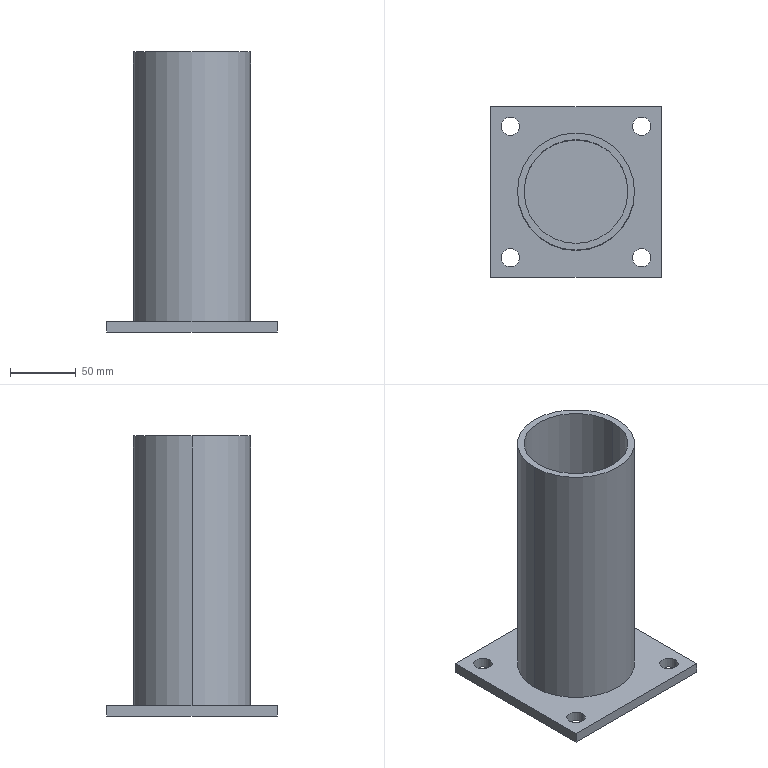Part | SolidWorks | features Extrusion 1, WeldMemberFeat 1, WeldmentFeature 1 | 2 solids | 20 faces | box 130 x 130 x 213 mm | volume 400765 mm3 | cylinder 12 | plane 8 | commonest cylinder face diameters 14 x8 79 x2 89 x2
STEP:
#1=CARTESIAN_POINT('',(-57.,-50.,8.));
#2=VERTEX_POINT('',#1);
#3=CARTESIAN_POINT('',(-43.,-50.,8.));
#4=VERTEX_POINT('',#3);
#5=CARTESIAN_POINT('',(-50.,-50.,8.));
#6=DIRECTION('',(0.,0.,1.));
#7=DIRECTION('',(-1.,0.,0.));
#8=AXIS2_PLACEMENT_3D('',#5,#6,#7);
#9=CIRCLE('',#8,7.);
#10=EDGE_CURVE('',#2,#4,#9,.T.);
#11=ORIENTED_EDGE('',*,*,#10,.T.);
#12=CARTESIAN_POINT('',(-43.,-50.,0.));
#13=VERTEX_POINT('',#12);
#14=CARTESIAN_POINT('',(-43.,-50.,8.));
#15=DIRECTION('',(0.,0.,-1.));
#16=VECTOR('',#15,1000.);
#17=LINE('',#14,#16);
#18=EDGE_CURVE('',#4,#13,#17,.T.);
#19=ORIENTED_EDGE('',*,*,#18,.T.);
#20=CARTESIAN_POINT('',(-57.,-50.,0.));
#21=VERTEX_POINT('',#20);
#22=CARTESIAN_POINT('',(-50.,-50.,0.));
#23=DIRECTION('',(0.,0.,1.));
#24=DIRECTION('',(-1.,0.,0.));
#25=AXIS2_PLACEMENT_3D('',#22,#23,#24);
#26=CIRCLE('',#25,7.);
#27=EDGE_CURVE('',#21,#13,#26,.T.);
#28=ORIENTED_EDGE('',*,*,#27,.F.);
#29=CARTESIAN_POINT('',(-57.,-50.,8.));
#30=DIRECTION('',(0.,0.,-1.));
#31=VECTOR('',#30,1000.);
#32=LINE('',#29,#31);
#33=EDGE_CURVE('',#2,#21,#32,.T.);
#34=ORIENTED_EDGE('',*,*,#33,.F.);
#35=EDGE_LOOP('',(#11,#19,#28,#34));
#36=FACE_OUTER_BOUND('',#35,.T.);
#37=CARTESIAN_POINT('',(-50.,-50.,8.));
#38=DIRECTION('',(0.,0.,-1.));
#39=DIRECTION('',(-1.,0.,0.));
#40=AXIS2_PLACEMENT_3D('',#37,#38,#39);
#41=CYLINDRICAL_SURFACE('',#40,7.);
#42=ADVANCED_FACE('',(#36),#41,.F.);
#43=CARTESIAN_POINT('',(43.,-50.,8.));
#44=VERTEX_POINT('',#43);
#45=CARTESIAN_POINT('',(57.,-50.,8.));
#46=VERTEX_POINT('',#45);
#47=CARTESIAN_POINT('',(50.,-50.,8.));
#48=DIRECTION('',(0.,0.,1.));
#49=DIRECTION('',(1.,0.,0.));
#50=AXIS2_PLACEMENT_3D('',#47,#48,#49);
#51=CIRCLE('',#50,7.);
#52=EDGE_CURVE('',#44,#46,#51,.T.);
#53=ORIENTED_EDGE('',*,*,#52,.T.);
#54=CARTESIAN_POINT('',(57.,-50.,0.));
#55=VERTEX_POINT('',#54);
#56=CARTESIAN_POINT('',(57.,-50.,8.));
#57=DIRECTION('',(0.,0.,-1.));
#58=VECTOR('',#57,1000.);
#59=LINE('',#56,#58);
#60=EDGE_CURVE('',#46,#55,#59,.T.);
#61=ORIENTED_EDGE('',*,*,#60,.T.);
#62=CARTESIAN_POINT('',(43.,-50.,0.));
#63=VERTEX_POINT('',#62);
#64=CARTESIAN_POINT('',(50.,-50.,0.));
#65=DIRECTION('',(0.,0.,1.));
#66=DIRECTION('',(1.,0.,0.));
#67=AXIS2_PLACEMENT_3D('',#64,#65,#66);
#68=CIRCLE('',#67,7.);
#69=EDGE_CURVE('',#63,#55,#68,.T.);
#70=ORIENTED_EDGE('',*,*,#69,.F.);
#71=CARTESIAN_POINT('',(43.,-50.,8.));
#72=DIRECTION('',(0.,0.,-1.));
#73=VECTOR('',#72,1000.);
#74=LINE('',#71,#73);
#75=EDGE_CURVE('',#44,#63,#74,.T.);
#76=ORIENTED_EDGE('',*,*,#75,.F.);
#77=EDGE_LOOP('',(#53,#61,#70,#76));
#78=FACE_OUTER_BOUND('',#77,.T.);
#79=CARTESIAN_POINT('',(50.,-50.,8.));
#80=DIRECTION('',(0.,0.,-1.));
#81=DIRECTION('',(-1.,0.,0.));
#82=AXIS2_PLACEMENT_3D('',#79,#80,#81);
#83=CYLINDRICAL_SURFACE('',#82,7.);
#84=ADVANCED_FACE('',(#78),#83,.F.);
#85=CARTESIAN_POINT('',(43.,50.,8.));
#86=VERTEX_POINT('',#85);
#87=CARTESIAN_POINT('',(57.,50.,8.));
#88=VERTEX_POINT('',#87);
#89=CARTESIAN_POINT('',(50.,50.,8.));
#90=DIRECTION('',(0.,0.,1.));
#91=DIRECTION('',(-1.,0.,0.));
#92=AXIS2_PLACEMENT_3D('',#89,#90,#91);
#93=CIRCLE('',#92,7.);
#94=EDGE_CURVE('',#86,#88,#93,.T.);
#95=ORIENTED_EDGE('',*,*,#94,.T.);
#96=CARTESIAN_POINT('',(57.,50.,0.));
#97=VERTEX_POINT('',#96);
#98=CARTESIAN_POINT('',(57.,50.,8.));
#99=DIRECTION('',(0.,0.,-1.));
#100=VECTOR('',#99,1000.);
#101=LINE('',#98,#100);
#102=EDGE_CURVE('',#88,#97,#101,.T.);
#103=ORIENTED_EDGE('',*,*,#102,.T.);
#104=CARTESIAN_POINT('',(43.,50.,0.));
#105=VERTEX_POINT('',#104);
#106=CARTESIAN_POINT('',(50.,50.,0.));
#107=DIRECTION('',(0.,0.,1.));
#108=DIRECTION('',(-1.,0.,0.));
#109=AXIS2_PLACEMENT_3D('',#106,#107,#108);
#110=CIRCLE('',#109,7.);
#111=EDGE_CURVE('',#105,#97,#110,.T.);
#112=ORIENTED_EDGE('',*,*,#111,.F.);
#113=CARTESIAN_POINT('',(43.,50.,8.));
#114=DIRECTION('',(0.,0.,-1.));
#115=VECTOR('',#114,1000.);
#116=LINE('',#113,#115);
#117=EDGE_CURVE('',#86,#105,#116,.T.);
#118=ORIENTED_EDGE('',*,*,#117,.F.);
#119=EDGE_LOOP('',(#95,#103,#112,#118));
#120=FACE_OUTER_BOUND('',#119,.T.);
#121=CARTESIAN_POINT('',(50.,50.,8.));
#122=DIRECTION('',(0.,0.,-1.));
#123=DIRECTION('',(-1.,0.,0.));
#124=AXIS2_PLACEMENT_3D('',#121,#122,#123);
#125=CYLINDRICAL_SURFACE('',#124,7.);
#126=ADVANCED_FACE('',(#120),#125,.F.);
#127=CARTESIAN_POINT('',(-57.,50.,8.));
#128=VERTEX_POINT('',#127);
#129=CARTESIAN_POINT('',(-43.,50.,8.));
#130=VERTEX_POINT('',#129);
#131=CARTESIAN_POINT('',(-50.,50.,8.));
#132=DIRECTION('',(0.,0.,1.));
#133=DIRECTION('',(1.,0.,0.));
#134=AXIS2_PLACEMENT_3D('',#131,#132,#133);
#135=CIRCLE('',#134,7.);
#136=EDGE_CURVE('',#128,#130,#135,.T.);
#137=ORIENTED_EDGE('',*,*,#136,.T.);
#138=CARTESIAN_POINT('',(-43.,50.,0.));
#139=VERTEX_POINT('',#138);
#140=CARTESIAN_POINT('',(-43.,50.,8.));
#141=DIRECTION('',(0.,0.,-1.));
#142=VECTOR('',#141,1000.);
#143=LINE('',#140,#142);
#144=EDGE_CURVE('',#130,#139,#143,.T.);
#145=ORIENTED_EDGE('',*,*,#144,.T.);
#146=CARTESIAN_POINT('',(-57.,50.,0.));
#147=VERTEX_POINT('',#146);
#148=CARTESIAN_POINT('',(-50.,50.,0.));
#149=DIRECTION('',(0.,0.,1.));
#150=DIRECTION('',(1.,0.,0.));
#151=AXIS2_PLACEMENT_3D('',#148,#149,#150);
#152=CIRCLE('',#151,7.);
#153=EDGE_CURVE('',#147,#139,#152,.T.);
#154=ORIENTED_EDGE('',*,*,#153,.F.);
#155=CARTESIAN_POINT('',(-57.,50.,8.));
#156=DIRECTION('',(0.,0.,-1.));
#157=VECTOR('',#156,1000.);
#158=LINE('',#155,#157);
#159=EDGE_CURVE('',#128,#147,#158,.T.);
#160=ORIENTED_EDGE('',*,*,#159,.F.);
#161=EDGE_LOOP('',(#137,#145,#154,#160));
#162=FACE_OUTER_BOUND('',#161,.T.);
#163=CARTESIAN_POINT('',(-50.,50.,8.));
#164=DIRECTION('',(0.,0.,-1.));
#165=DIRECTION('',(-1.,0.,0.));
#166=AXIS2_PLACEMENT_3D('',#163,#164,#165);
#167=CYLINDRICAL_SURFACE('',#166,7.);
#168=ADVANCED_FACE('',(#162),#167,.F.);
#169=ORIENTED_EDGE('',*,*,#52,.F.);
#170=CARTESIAN_POINT('',(50.,-50.,8.));
#171=DIRECTION('',(0.,0.,1.));
#172=DIRECTION('',(1.,0.,0.));
#173=AXIS2_PLACEMENT_3D('',#170,#171,#172);
#174=CIRCLE('',#173,7.);
#175=EDGE_CURVE('',#46,#44,#174,.T.);
#176=ORIENTED_EDGE('',*,*,#175,.F.);
#177=EDGE_LOOP('',(#169,#176));
#178=FACE_BOUND('',#177,.T.);
#179=ORIENTED_EDGE('',*,*,#136,.F.);
#180=CARTESIAN_POINT('',(-50.,50.,8.));
#181=DIRECTION('',(0.,0.,1.));
#182=DIRECTION('',(1.,0.,0.));
#183=AXIS2_PLACEMENT_3D('',#180,#181,#182);
#184=CIRCLE('',#183,7.);
#185=EDGE_CURVE('',#130,#128,#184,.T.);
#186=ORIENTED_EDGE('',*,*,#185,.F.);
#187=EDGE_LOOP('',(#179,#186));
#188=FACE_BOUND('',#187,.T.);
#189=CARTESIAN_POINT('',(-65.,65.,8.));
#190=VERTEX_POINT('',#189);
#191=CARTESIAN_POINT('',(-65.,-65.,8.));
#192=VERTEX_POINT('',#191);
#193=CARTESIAN_POINT('',(-65.,-65.,8.));
#194=DIRECTION('',(0.,-1.,0.));
#195=VECTOR('',#194,1000.);
#196=LINE('',#193,#195);
#197=EDGE_CURVE('',#190,#192,#196,.T.);
#198=ORIENTED_EDGE('',*,*,#197,.T.);
#199=CARTESIAN_POINT('',(65.,-65.,8.));
#200=VERTEX_POINT('',#199);
#201=CARTESIAN_POINT('',(65.,-65.,8.));
#202=DIRECTION('',(1.,0.,0.));
#203=VECTOR('',#202,1000.);
#204=LINE('',#201,#203);
#205=EDGE_CURVE('',#192,#200,#204,.T.);
#206=ORIENTED_EDGE('',*,*,#205,.T.);
#207=CARTESIAN_POINT('',(65.,65.,8.));
#208=VERTEX_POINT('',#207);
#209=CARTESIAN_POINT('',(65.,-65.,8.));
#210=DIRECTION('',(0.,1.,0.));
#211=VECTOR('',#210,1000.);
#212=LINE('',#209,#211);
#213=EDGE_CURVE('',#200,#208,#212,.T.);
#214=ORIENTED_EDGE('',*,*,#213,.T.);
#215=CARTESIAN_POINT('',(65.,65.,8.));
#216=DIRECTION('',(-1.,0.,0.));
#217=VECTOR('',#216,1000.);
#218=LINE('',#215,#217);
#219=EDGE_CURVE('',#208,#190,#218,.T.);
#220=ORIENTED_EDGE('',*,*,#219,.T.);
#221=EDGE_LOOP('',(#198,#206,#214,#220));
#222=FACE_OUTER_BOUND('',#221,.T.);
#223=ORIENTED_EDGE('',*,*,#94,.F.);
#224=CARTESIAN_POINT('',(50.,50.,8.));
#225=DIRECTION('',(0.,0.,1.));
#226=DIRECTION('',(-1.,0.,0.));
#227=AXIS2_PLACEMENT_3D('',#224,#225,#226);
#228=CIRCLE('',#227,7.);
#229=EDGE_CURVE('',#88,#86,#228,.T.);
#230=ORIENTED_EDGE('',*,*,#229,.F.);
#231=EDGE_LOOP('',(#223,#230));
#232=FACE_BOUND('',#231,.T.);
#233=ORIENTED_EDGE('',*,*,#10,.F.);
#234=CARTESIAN_POINT('',(-50.,-50.,8.));
#235=DIRECTION('',(0.,0.,1.));
#236=DIRECTION('',(-1.,0.,0.));
#237=AXIS2_PLACEMENT_3D('',#234,#235,#236);
#238=CIRCLE('',#237,7.);
#239=EDGE_CURVE('',#4,#2,#238,.T.);
#240=ORIENTED_EDGE('',*,*,#239,.F.);
#241=EDGE_LOOP('',(#233,#240));
#242=FACE_BOUND('',#241,.T.);
#243=CARTESIAN_POINT('',(0.,0.,8.));
#244=DIRECTION('',(0.,0.,1.));
#245=DIRECTION('',(1.,0.,0.));
#246=AXIS2_PLACEMENT_3D('',#243,#244,#245);
#247=PLANE('',#246);
#248=ADVANCED_FACE('',(#178,#188,#222,#232,#242),#247,.T.);
#249=CARTESIAN_POINT('',(-65.,65.,0.));
#250=VERTEX_POINT('',#249);
#251=CARTESIAN_POINT('',(-65.,-65.,0.));
#252=VERTEX_POINT('',#251);
#253=CARTESIAN_POINT('',(-65.,-65.,0.));
#254=DIRECTION('',(0.,-1.,0.));
#255=VECTOR('',#254,1000.);
#256=LINE('',#253,#255);
#257=EDGE_CURVE('',#250,#252,#256,.T.);
#258=ORIENTED_EDGE('',*,*,#257,.F.);
#259=CARTESIAN_POINT('',(65.,65.,0.));
#260=VERTEX_POINT('',#259);
#261=CARTESIAN_POINT('',(65.,65.,0.));
#262=DIRECTION('',(-1.,0.,0.));
#263=VECTOR('',#262,1000.);
#264=LINE('',#261,#263);
#265=EDGE_CURVE('',#260,#250,#264,.T.);
#266=ORIENTED_EDGE('',*,*,#265,.F.);
#267=CARTESIAN_POINT('',(65.,-65.,0.));
#268=VERTEX_POINT('',#267);
#269=CARTESIAN_POINT('',(65.,-65.,0.));
#270=DIRECTION('',(0.,1.,0.));
#271=VECTOR('',#270,1000.);
#272=LINE('',#269,#271);
#273=EDGE_CURVE('',#268,#260,#272,.T.);
#274=ORIENTED_EDGE('',*,*,#273,.F.);
#275=CARTESIAN_POINT('',(65.,-65.,0.));
#276=DIRECTION('',(1.,0.,0.));
#277=VECTOR('',#276,1000.);
#278=LINE('',#275,#277);
#279=EDGE_CURVE('',#252,#268,#278,.T.);
#280=ORIENTED_EDGE('',*,*,#279,.F.);
#281=EDGE_LOOP('',(#258,#266,#274,#280));
#282=FACE_OUTER_BOUND('',#281,.T.);
#283=ORIENTED_EDGE('',*,*,#153,.T.);
#284=CARTESIAN_POINT('',(-50.,50.,0.));
#285=DIRECTION('',(0.,0.,1.));
#286=DIRECTION('',(1.,0.,0.));
#287=AXIS2_PLACEMENT_3D('',#284,#285,#286);
#288=CIRCLE('',#287,7.);
#289=EDGE_CURVE('',#139,#147,#288,.T.);
#290=ORIENTED_EDGE('',*,*,#289,.T.);
#291=EDGE_LOOP('',(#283,#290));
#292=FACE_BOUND('',#291,.T.);
#293=ORIENTED_EDGE('',*,*,#111,.T.);
#294=CARTESIAN_POINT('',(50.,50.,0.));
#295=DIRECTION('',(0.,0.,1.));
#296=DIRECTION('',(-1.,0.,0.));
#297=AXIS2_PLACEMENT_3D('',#294,#295,#296);
#298=CIRCLE('',#297,7.);
#299=EDGE_CURVE('',#97,#105,#298,.T.);
#300=ORIENTED_EDGE('',*,*,#299,.T.);
#301=EDGE_LOOP('',(#293,#300));
#302=FACE_BOUND('',#301,.T.);
#303=ORIENTED_EDGE('',*,*,#69,.T.);
#304=CARTESIAN_POINT('',(50.,-50.,0.));
#305=DIRECTION('',(0.,0.,1.));
#306=DIRECTION('',(1.,0.,0.));
#307=AXIS2_PLACEMENT_3D('',#304,#305,#306);
#308=CIRCLE('',#307,7.);
#309=EDGE_CURVE('',#55,#63,#308,.T.);
#310=ORIENTED_EDGE('',*,*,#309,.T.);
#311=EDGE_LOOP('',(#303,#310));
#312=FACE_BOUND('',#311,.T.);
#313=ORIENTED_EDGE('',*,*,#27,.T.);
#314=CARTESIAN_POINT('',(-50.,-50.,0.));
#315=DIRECTION('',(0.,0.,1.));
#316=DIRECTION('',(-1.,0.,0.));
#317=AXIS2_PLACEMENT_3D('',#314,#315,#316);
#318=CIRCLE('',#317,7.);
#319=EDGE_CURVE('',#13,#21,#318,.T.);
#320=ORIENTED_EDGE('',*,*,#319,.T.);
#321=EDGE_LOOP('',(#313,#320));
#322=FACE_BOUND('',#321,.T.);
#323=CARTESIAN_POINT('',(0.,0.,0.));
#324=DIRECTION('',(0.,0.,1.));
#325=DIRECTION('',(1.,0.,0.));
#326=AXIS2_PLACEMENT_3D('',#323,#324,#325);
#327=PLANE('',#326);
#328=ADVANCED_FACE('',(#282,#292,#302,#312,#322),#327,.F.);
#329=ORIENTED_EDGE('',*,*,#257,.T.);
#330=CARTESIAN_POINT('',(-65.,-65.,8.));
#331=DIRECTION('',(0.,0.,-1.));
#332=VECTOR('',#331,1000.);
#333=LINE('',#330,#332);
#334=EDGE_CURVE('',#192,#252,#333,.T.);
#335=ORIENTED_EDGE('',*,*,#334,.F.);
#336=ORIENTED_EDGE('',*,*,#197,.F.);
#337=CARTESIAN_POINT('',(-65.,65.,8.));
#338=DIRECTION('',(0.,0.,-1.));
#339=VECTOR('',#338,1000.);
#340=LINE('',#337,#339);
#341=EDGE_CURVE('',#190,#250,#340,.T.);
#342=ORIENTED_EDGE('',*,*,#341,.T.);
#343=EDGE_LOOP('',(#329,#335,#336,#342));
#344=FACE_OUTER_BOUND('',#343,.T.);
#345=CARTESIAN_POINT('',(-65.,-65.,8.));
#346=DIRECTION('',(1.,0.,0.));
#347=DIRECTION('',(0.,0.,-1.));
#348=AXIS2_PLACEMENT_3D('',#345,#346,#347);
#349=PLANE('',#348);
#350=ADVANCED_FACE('',(#344),#349,.F.);
#351=ORIENTED_EDGE('',*,*,#279,.T.);
#352=CARTESIAN_POINT('',(65.,-65.,8.));
#353=DIRECTION('',(0.,0.,-1.));
#354=VECTOR('',#353,1000.);
#355=LINE('',#352,#354);
#356=EDGE_CURVE('',#200,#268,#355,.T.);
#357=ORIENTED_EDGE('',*,*,#356,.F.);
#358=ORIENTED_EDGE('',*,*,#205,.F.);
#359=ORIENTED_EDGE('',*,*,#334,.T.);
#360=EDGE_LOOP('',(#351,#357,#358,#359));
#361=FACE_OUTER_BOUND('',#360,.T.);
#362=CARTESIAN_POINT('',(65.,-65.,8.));
#363=DIRECTION('',(0.,1.,0.));
#364=DIRECTION('',(-1.,0.,0.));
#365=AXIS2_PLACEMENT_3D('',#362,#363,#364);
#366=PLANE('',#365);
#367=ADVANCED_FACE('',(#361),#366,.F.);
#368=ORIENTED_EDGE('',*,*,#273,.T.);
#369=CARTESIAN_POINT('',(65.,65.,8.));
#370=DIRECTION('',(0.,0.,-1.));
#371=VECTOR('',#370,1000.);
#372=LINE('',#369,#371);
#373=EDGE_CURVE('',#208,#260,#372,.T.);
#374=ORIENTED_EDGE('',*,*,#373,.F.);
#375=ORIENTED_EDGE('',*,*,#213,.F.);
#376=ORIENTED_EDGE('',*,*,#356,.T.);
#377=EDGE_LOOP('',(#368,#374,#375,#376));
#378=FACE_OUTER_BOUND('',#377,.T.);
#379=CARTESIAN_POINT('',(65.,-65.,8.));
#380=DIRECTION('',(-1.,0.,0.));
#381=DIRECTION('',(0.,0.,1.));
#382=AXIS2_PLACEMENT_3D('',#379,#380,#381);
#383=PLANE('',#382);
#384=ADVANCED_FACE('',(#378),#383,.F.);
#385=ORIENTED_EDGE('',*,*,#265,.T.);
#386=ORIENTED_EDGE('',*,*,#341,.F.);
#387=ORIENTED_EDGE('',*,*,#219,.F.);
#388=ORIENTED_EDGE('',*,*,#373,.T.);
#389=EDGE_LOOP('',(#385,#386,#387,#388));
#390=FACE_OUTER_BOUND('',#389,.T.);
#391=CARTESIAN_POINT('',(65.,65.,8.));
#392=DIRECTION('',(0.,-1.,0.));
#393=DIRECTION('',(0.,0.,-1.));
#394=AXIS2_PLACEMENT_3D('',#391,#392,#393);
#395=PLANE('',#394);
#396=ADVANCED_FACE('',(#390),#395,.F.);
#397=ORIENTED_EDGE('',*,*,#144,.F.);
#398=ORIENTED_EDGE('',*,*,#185,.T.);
#399=ORIENTED_EDGE('',*,*,#159,.T.);
#400=ORIENTED_EDGE('',*,*,#289,.F.);
#401=EDGE_LOOP('',(#397,#398,#399,#400));
#402=FACE_OUTER_BOUND('',#401,.T.);
#403=CARTESIAN_POINT('',(-50.,50.,8.));
#404=DIRECTION('',(0.,0.,-1.));
#405=DIRECTION('',(-1.,0.,0.));
#406=AXIS2_PLACEMENT_3D('',#403,#404,#405);
#407=CYLINDRICAL_SURFACE('',#406,7.);
#408=ADVANCED_FACE('',(#402),#407,.F.);
#409=ORIENTED_EDGE('',*,*,#102,.F.);
#410=ORIENTED_EDGE('',*,*,#229,.T.);
#411=ORIENTED_EDGE('',*,*,#117,.T.);
#412=ORIENTED_EDGE('',*,*,#299,.F.);
#413=EDGE_LOOP('',(#409,#410,#411,#412));
#414=FACE_OUTER_BOUND('',#413,.T.);
#415=CARTESIAN_POINT('',(50.,50.,8.));
#416=DIRECTION('',(0.,0.,-1.));
#417=DIRECTION('',(-1.,0.,0.));
#418=AXIS2_PLACEMENT_3D('',#415,#416,#417);
#419=CYLINDRICAL_SURFACE('',#418,7.);
#420=ADVANCED_FACE('',(#414),#419,.F.);
#421=ORIENTED_EDGE('',*,*,#60,.F.);
#422=ORIENTED_EDGE('',*,*,#175,.T.);
#423=ORIENTED_EDGE('',*,*,#75,.T.);
#424=ORIENTED_EDGE('',*,*,#309,.F.);
#425=EDGE_LOOP('',(#421,#422,#423,#424));
#426=FACE_OUTER_BOUND('',#425,.T.);
#427=CARTESIAN_POINT('',(50.,-50.,8.));
#428=DIRECTION('',(0.,0.,-1.));
#429=DIRECTION('',(-1.,0.,0.));
#430=AXIS2_PLACEMENT_3D('',#427,#428,#429);
#431=CYLINDRICAL_SURFACE('',#430,7.);
#432=ADVANCED_FACE('',(#426),#431,.F.);
#433=ORIENTED_EDGE('',*,*,#18,.F.);
#434=ORIENTED_EDGE('',*,*,#239,.T.);
#435=ORIENTED_EDGE('',*,*,#33,.T.);
#436=ORIENTED_EDGE('',*,*,#319,.F.);
#437=EDGE_LOOP('',(#433,#434,#435,#436));
#438=FACE_OUTER_BOUND('',#437,.T.);
#439=CARTESIAN_POINT('',(-50.,-50.,8.));
#440=DIRECTION('',(0.,0.,-1.));
#441=DIRECTION('',(-1.,0.,0.));
#442=AXIS2_PLACEMENT_3D('',#439,#440,#441);
#443=CYLINDRICAL_SURFACE('',#442,7.);
#444=ADVANCED_FACE('',(#438),#443,.F.);
#445=CLOSED_SHELL('',(#42,#84,#126,#168,#248,#328,#350,#367,#384,#396,#408,#420,#432,#444));
#446=MANIFOLD_SOLID_BREP('',#445);
#447=CARTESIAN_POINT('',(44.5,0.,213.));
#448=VERTEX_POINT('',#447);
#449=CARTESIAN_POINT('',(-44.5,0.,213.));
#450=VERTEX_POINT('',#449);
#451=CARTESIAN_POINT('',(0.,0.,213.));
#452=DIRECTION('',(0.,0.,1.));
#453=DIRECTION('',(1.,0.,0.));
#454=AXIS2_PLACEMENT_3D('',#451,#452,#453);
#455=CIRCLE('',#454,44.5);
#456=EDGE_CURVE('',#448,#450,#455,.T.);
#457=ORIENTED_EDGE('',*,*,#456,.F.);
#458=CARTESIAN_POINT('',(44.5,0.,8.));
#459=VERTEX_POINT('',#458);
#460=CARTESIAN_POINT('',(44.5,0.,213.));
#461=DIRECTION('',(0.,0.,-1.));
#462=VECTOR('',#461,1000.);
#463=LINE('',#460,#462);
#464=EDGE_CURVE('',#448,#459,#463,.T.);
#465=ORIENTED_EDGE('',*,*,#464,.T.);
#466=CARTESIAN_POINT('',(-44.5,0.,8.));
#467=VERTEX_POINT('',#466);
#468=CARTESIAN_POINT('',(0.,0.,8.));
#469=DIRECTION('',(0.,0.,1.));
#470=DIRECTION('',(1.,0.,0.));
#471=AXIS2_PLACEMENT_3D('',#468,#469,#470);
#472=CIRCLE('',#471,44.5);
#473=EDGE_CURVE('',#459,#467,#472,.T.);
#474=ORIENTED_EDGE('',*,*,#473,.T.);
#475=CARTESIAN_POINT('',(-44.5,0.,213.));
#476=DIRECTION('',(0.,0.,-1.));
#477=VECTOR('',#476,1000.);
#478=LINE('',#475,#477);
#479=EDGE_CURVE('',#450,#467,#478,.T.);
#480=ORIENTED_EDGE('',*,*,#479,.F.);
#481=EDGE_LOOP('',(#457,#465,#474,#480));
#482=FACE_OUTER_BOUND('',#481,.T.);
#483=CARTESIAN_POINT('',(0.,0.,213.));
#484=DIRECTION('',(0.,0.,-1.));
#485=DIRECTION('',(-1.,0.,0.));
#486=AXIS2_PLACEMENT_3D('',#483,#484,#485);
#487=CYLINDRICAL_SURFACE('',#486,44.5);
#488=ADVANCED_FACE('',(#482),#487,.T.);
#489=CARTESIAN_POINT('',(-39.5,0.,213.));
#490=VERTEX_POINT('',#489);
#491=CARTESIAN_POINT('',(39.5,0.,213.));
#492=VERTEX_POINT('',#491);
#493=CARTESIAN_POINT('',(0.,0.,213.));
#494=DIRECTION('',(0.,0.,1.));
#495=DIRECTION('',(1.,0.,0.));
#496=AXIS2_PLACEMENT_3D('',#493,#494,#495);
#497=CIRCLE('',#496,39.5);
#498=EDGE_CURVE('',#490,#492,#497,.T.);
#499=ORIENTED_EDGE('',*,*,#498,.T.);
#500=CARTESIAN_POINT('',(39.5,0.,8.));
#501=VERTEX_POINT('',#500);
#502=CARTESIAN_POINT('',(39.5,0.,213.));
#503=DIRECTION('',(0.,0.,-1.));
#504=VECTOR('',#503,1000.);
#505=LINE('',#502,#504);
#506=EDGE_CURVE('',#492,#501,#505,.T.);
#507=ORIENTED_EDGE('',*,*,#506,.T.);
#508=CARTESIAN_POINT('',(-39.5,0.,8.));
#509=VERTEX_POINT('',#508);
#510=CARTESIAN_POINT('',(0.,0.,8.));
#511=DIRECTION('',(0.,0.,1.));
#512=DIRECTION('',(1.,0.,0.));
#513=AXIS2_PLACEMENT_3D('',#510,#511,#512);
#514=CIRCLE('',#513,39.5);
#515=EDGE_CURVE('',#509,#501,#514,.T.);
#516=ORIENTED_EDGE('',*,*,#515,.F.);
#517=CARTESIAN_POINT('',(-39.5,0.,213.));
#518=DIRECTION('',(0.,0.,-1.));
#519=VECTOR('',#518,1000.);
#520=LINE('',#517,#519);
#521=EDGE_CURVE('',#490,#509,#520,.T.);
#522=ORIENTED_EDGE('',*,*,#521,.F.);
#523=EDGE_LOOP('',(#499,#507,#516,#522));
#524=FACE_OUTER_BOUND('',#523,.T.);
#525=CARTESIAN_POINT('',(0.,0.,213.));
#526=DIRECTION('',(0.,0.,-1.));
#527=DIRECTION('',(-1.,0.,0.));
#528=AXIS2_PLACEMENT_3D('',#525,#526,#527);
#529=CYLINDRICAL_SURFACE('',#528,39.5);
#530=ADVANCED_FACE('',(#524),#529,.F.);
#531=ORIENTED_EDGE('',*,*,#506,.F.);
#532=CARTESIAN_POINT('',(0.,0.,213.));
#533=DIRECTION('',(0.,0.,1.));
#534=DIRECTION('',(1.,0.,0.));
#535=AXIS2_PLACEMENT_3D('',#532,#533,#534);
#536=CIRCLE('',#535,39.5);
#537=EDGE_CURVE('',#492,#490,#536,.T.);
#538=ORIENTED_EDGE('',*,*,#537,.T.);
#539=ORIENTED_EDGE('',*,*,#521,.T.);
#540=CARTESIAN_POINT('',(0.,0.,8.));
#541=DIRECTION('',(0.,0.,1.));
#542=DIRECTION('',(1.,0.,0.));
#543=AXIS2_PLACEMENT_3D('',#540,#541,#542);
#544=CIRCLE('',#543,39.5);
#545=EDGE_CURVE('',#501,#509,#544,.T.);
#546=ORIENTED_EDGE('',*,*,#545,.F.);
#547=EDGE_LOOP('',(#531,#538,#539,#546));
#548=FACE_OUTER_BOUND('',#547,.T.);
#549=CARTESIAN_POINT('',(0.,0.,213.));
#550=DIRECTION('',(0.,0.,-1.));
#551=DIRECTION('',(-1.,0.,0.));
#552=AXIS2_PLACEMENT_3D('',#549,#550,#551);
#553=CYLINDRICAL_SURFACE('',#552,39.5);
#554=ADVANCED_FACE('',(#548),#553,.F.);
#555=ORIENTED_EDGE('',*,*,#464,.F.);
#556=CARTESIAN_POINT('',(0.,0.,213.));
#557=DIRECTION('',(0.,0.,1.));
#558=DIRECTION('',(1.,0.,0.));
#559=AXIS2_PLACEMENT_3D('',#556,#557,#558);
#560=CIRCLE('',#559,44.5);
#561=EDGE_CURVE('',#450,#448,#560,.T.);
#562=ORIENTED_EDGE('',*,*,#561,.F.);
#563=ORIENTED_EDGE('',*,*,#479,.T.);
#564=CARTESIAN_POINT('',(0.,0.,8.));
#565=DIRECTION('',(0.,0.,1.));
#566=DIRECTION('',(1.,0.,0.));
#567=AXIS2_PLACEMENT_3D('',#564,#565,#566);
#568=CIRCLE('',#567,44.5);
#569=EDGE_CURVE('',#467,#459,#568,.T.);
#570=ORIENTED_EDGE('',*,*,#569,.T.);
#571=EDGE_LOOP('',(#555,#562,#563,#570));
#572=FACE_OUTER_BOUND('',#571,.T.);
#573=CARTESIAN_POINT('',(0.,0.,213.));
#574=DIRECTION('',(0.,0.,-1.));
#575=DIRECTION('',(-1.,0.,0.));
#576=AXIS2_PLACEMENT_3D('',#573,#574,#575);
#577=CYLINDRICAL_SURFACE('',#576,44.5);
#578=ADVANCED_FACE('',(#572),#577,.T.);
#579=ORIENTED_EDGE('',*,*,#498,.F.);
#580=ORIENTED_EDGE('',*,*,#537,.F.);
#581=EDGE_LOOP('',(#579,#580));
#582=FACE_BOUND('',#581,.T.);
#583=ORIENTED_EDGE('',*,*,#561,.T.);
#584=ORIENTED_EDGE('',*,*,#456,.T.);
#585=EDGE_LOOP('',(#583,#584));
#586=FACE_OUTER_BOUND('',#585,.T.);
#587=CARTESIAN_POINT('',(0.,0.,213.));
#588=DIRECTION('',(0.,0.,1.));
#589=DIRECTION('',(1.,0.,0.));
#590=AXIS2_PLACEMENT_3D('',#587,#588,#589);
#591=PLANE('',#590);
#592=ADVANCED_FACE('',(#582,#586),#591,.T.);
#593=ORIENTED_EDGE('',*,*,#515,.T.);
#594=ORIENTED_EDGE('',*,*,#545,.T.);
#595=EDGE_LOOP('',(#593,#594));
#596=FACE_BOUND('',#595,.T.);
#597=ORIENTED_EDGE('',*,*,#569,.F.);
#598=ORIENTED_EDGE('',*,*,#473,.F.);
#599=EDGE_LOOP('',(#597,#598));
#600=FACE_OUTER_BOUND('',#599,.T.);
#601=CARTESIAN_POINT('',(0.,0.,8.));
#602=DIRECTION('',(0.,0.,1.));
#603=DIRECTION('',(1.,0.,0.));
#604=AXIS2_PLACEMENT_3D('',#601,#602,#603);
#605=PLANE('',#604);
#606=ADVANCED_FACE('',(#596,#600),#605,.F.);
#607=CLOSED_SHELL('',(#488,#530,#554,#578,#592,#606));
#608=MANIFOLD_SOLID_BREP('',#607);
#609=CARTESIAN_POINT('',(0.,0.,0.));
#610=DIRECTION('',(0.,0.,1.));
#611=DIRECTION('',(1.,0.,0.));
#612=AXIS2_PLACEMENT_3D('',#609,#610,#611);
#613=(LENGTH_UNIT()NAMED_UNIT(*)SI_UNIT(.MILLI.,.METRE.));
#614=UNCERTAINTY_MEASURE_WITH_UNIT(LENGTH_MEASURE(0.00001),#613,'','');
#615=(NAMED_UNIT(*)PLANE_ANGLE_UNIT()SI_UNIT($,.RADIAN.));
#616=(NAMED_UNIT(*)SI_UNIT($,.STERADIAN.)SOLID_ANGLE_UNIT());
#617=(GEOMETRIC_REPRESENTATION_CONTEXT(3)GLOBAL_UNCERTAINTY_ASSIGNED_CONTEXT((#614))GLOBAL_UNIT_ASSIGNED_CONTEXT((#613,#615,#616))REPRESENTATION_CONTEXT('',''));
#618=ADVANCED_BREP_SHAPE_REPRESENTATION('',(#446,#608,#612),#617);